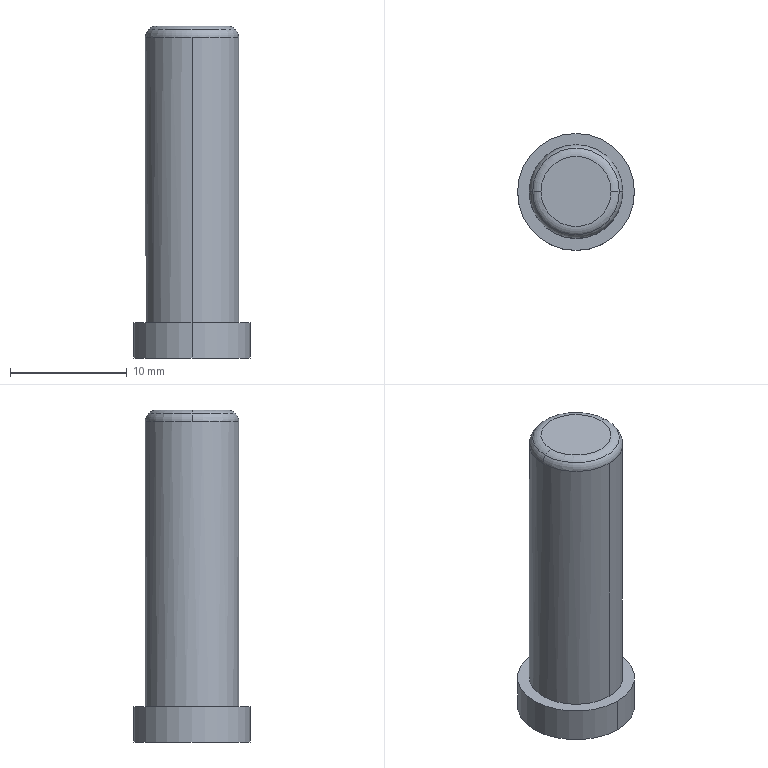Part | STEP file | 1_id1574_x_t | 1 solid | 11 faces | box 10 x 10 x 28.4 mm | volume 1507 mm3 | cylinder 4 | torus 4 | plane 3 | commonest cylinder face diameters 8 x2 10 x2
STEP:
#1=CARTESIAN_POINT('',(0.,0.,0.));
#2=DIRECTION('',(0.,0.,1.));
#3=DIRECTION('',(1.,0.,0.));
#4=AXIS2_PLACEMENT_3D('',#1,#2,#3);
#5=CARTESIAN_POINT('',(335.025,87.797,-28.4));
#6=VERTEX_POINT('',#5);
#7=CARTESIAN_POINT('',(335.025,87.797,-25.4));
#8=VERTEX_POINT('',#7);
#9=CARTESIAN_POINT('',(335.025,87.797,-28.4));
#10=DIRECTION('',(0.,0.,1.));
#11=VECTOR('',#10,1.);
#12=LINE('',#9,#11);
#13=CARTESIAN_POINT('',(335.025,92.797,-46.3));
#14=DIRECTION('',(0.,0.,1.));
#15=DIRECTION('',(0.,-1.,0.));
#16=AXIS2_PLACEMENT_3D('',#13,#14,#15);
#17=CYLINDRICAL_SURFACE('',#16,5.);
#18=CARTESIAN_POINT('',(6.283,17.9));
#19=DIRECTION('',(0.,1.));
#20=VECTOR('',#19,1.);
#21=LINE('',#18,#20);
#22=(GEOMETRIC_REPRESENTATION_CONTEXT(2)PARAMETRIC_REPRESENTATION_CONTEXT()REPRESENTATION_CONTEXT('',''));
#23=DEFINITIONAL_REPRESENTATION('',(#21),#22);
#24=PCURVE('',#17,#23);
#25=CARTESIAN_POINT('',(335.025,92.797,-46.3));
#26=DIRECTION('',(0.,0.,1.));
#27=DIRECTION('',(0.,-1.,0.));
#28=AXIS2_PLACEMENT_3D('',#25,#26,#27);
#29=CYLINDRICAL_SURFACE('',#28,5.);
#30=CARTESIAN_POINT('',(0.,17.9));
#31=DIRECTION('',(0.,1.));
#32=VECTOR('',#31,1.);
#33=LINE('',#30,#32);
#34=(GEOMETRIC_REPRESENTATION_CONTEXT(2)PARAMETRIC_REPRESENTATION_CONTEXT()REPRESENTATION_CONTEXT('',''));
#35=DEFINITIONAL_REPRESENTATION('',(#33),#34);
#36=PCURVE('',#29,#35);
#37=SURFACE_CURVE('',#12,(#24,#36),.PCURVE_S1.);
#38=EDGE_CURVE('',#6,#8,#37,.T.);
#39=ORIENTED_EDGE('',*,*,#38,.T.);
#40=CARTESIAN_POINT('',(335.025,97.797,-25.4));
#41=VERTEX_POINT('',#40);
#42=CARTESIAN_POINT('',(335.025,92.797,-25.4));
#43=DIRECTION('',(0.,0.,1.));
#44=DIRECTION('',(0.,1.,0.));
#45=AXIS2_PLACEMENT_3D('',#42,#43,#44);
#46=CIRCLE('',#45,5.);
#47=CARTESIAN_POINT('',(3.142,20.9));
#48=DIRECTION('',(1.,0.));
#49=VECTOR('',#48,1.);
#50=LINE('',#47,#49);
#51=(GEOMETRIC_REPRESENTATION_CONTEXT(2)PARAMETRIC_REPRESENTATION_CONTEXT()REPRESENTATION_CONTEXT('',''));
#52=DEFINITIONAL_REPRESENTATION('',(#50),#51);
#53=PCURVE('',#17,#52);
#54=CARTESIAN_POINT('',(335.025,92.797,-25.4));
#55=DIRECTION('',(0.,0.,1.));
#56=DIRECTION('',(-1.,0.,0.));
#57=AXIS2_PLACEMENT_3D('',#54,#55,#56);
#58=PLANE('',#57);
#59=CARTESIAN_POINT('',(0.,0.));
#60=DIRECTION('',(0.,-1.));
#61=AXIS2_PLACEMENT_2D('',#59,#60);
#62=CIRCLE('',#61,5.);
#63=(GEOMETRIC_REPRESENTATION_CONTEXT(2)PARAMETRIC_REPRESENTATION_CONTEXT()REPRESENTATION_CONTEXT('',''));
#64=DEFINITIONAL_REPRESENTATION('',(#62),#63);
#65=PCURVE('',#58,#64);
#66=SURFACE_CURVE('',#46,(#53,#65),.PCURVE_S1.);
#67=EDGE_CURVE('',#41,#8,#66,.T.);
#68=ORIENTED_EDGE('',*,*,#67,.F.);
#69=CARTESIAN_POINT('',(335.025,97.797,-28.4));
#70=VERTEX_POINT('',#69);
#71=CARTESIAN_POINT('',(335.025,97.797,-28.4));
#72=DIRECTION('',(0.,0.,-1.));
#73=VECTOR('',#72,1.);
#74=LINE('',#71,#73);
#75=CARTESIAN_POINT('',(3.142,17.9));
#76=DIRECTION('',(0.,-1.));
#77=VECTOR('',#76,1.);
#78=LINE('',#75,#77);
#79=(GEOMETRIC_REPRESENTATION_CONTEXT(2)PARAMETRIC_REPRESENTATION_CONTEXT()REPRESENTATION_CONTEXT('',''));
#80=DEFINITIONAL_REPRESENTATION('',(#78),#79);
#81=PCURVE('',#17,#80);
#82=CARTESIAN_POINT('',(3.142,17.9));
#83=DIRECTION('',(0.,-1.));
#84=VECTOR('',#83,1.);
#85=LINE('',#82,#84);
#86=(GEOMETRIC_REPRESENTATION_CONTEXT(2)PARAMETRIC_REPRESENTATION_CONTEXT()REPRESENTATION_CONTEXT('',''));
#87=DEFINITIONAL_REPRESENTATION('',(#85),#86);
#88=PCURVE('',#29,#87);
#89=SURFACE_CURVE('',#74,(#81,#88),.PCURVE_S1.);
#90=EDGE_CURVE('',#41,#70,#89,.T.);
#91=ORIENTED_EDGE('',*,*,#90,.T.);
#92=CARTESIAN_POINT('',(335.025,92.797,-28.4));
#93=DIRECTION('',(0.,0.,-1.));
#94=DIRECTION('',(0.,-1.,0.));
#95=AXIS2_PLACEMENT_3D('',#92,#93,#94);
#96=CIRCLE('',#95,5.);
#97=CARTESIAN_POINT('',(6.283,17.9));
#98=DIRECTION('',(-1.,0.));
#99=VECTOR('',#98,1.);
#100=LINE('',#97,#99);
#101=(GEOMETRIC_REPRESENTATION_CONTEXT(2)PARAMETRIC_REPRESENTATION_CONTEXT()REPRESENTATION_CONTEXT('',''));
#102=DEFINITIONAL_REPRESENTATION('',(#100),#101);
#103=PCURVE('',#17,#102);
#104=CARTESIAN_POINT('',(335.025,92.797,-28.4));
#105=DIRECTION('',(0.,0.,1.));
#106=DIRECTION('',(-1.,0.,0.));
#107=AXIS2_PLACEMENT_3D('',#104,#105,#106);
#108=PLANE('',#107);
#109=CARTESIAN_POINT('',(0.,5.));
#110=CARTESIAN_POINT('',(8.66,5.));
#111=CARTESIAN_POINT('',(4.33,-2.5));
#112=CARTESIAN_POINT('',(0.,-10.));
#113=CARTESIAN_POINT('',(-4.33,-2.5));
#114=CARTESIAN_POINT('',(-8.66,5.));
#115=CARTESIAN_POINT('',(0.,5.));
#116=(BOUNDED_CURVE()B_SPLINE_CURVE(2,(#109,#110,#111,#112,#113,#114,#115),.UNSPECIFIED.,.T.,.F.)B_SPLINE_CURVE_WITH_KNOTS((1,2,2,2,2,1),(-2.094,0.,2.094,4.189,6.283,8.378),.UNSPECIFIED.)CURVE()GEOMETRIC_REPRESENTATION_ITEM()RATIONAL_B_SPLINE_CURVE((1.,0.5,1.,0.5,1.,0.5,1.))REPRESENTATION_ITEM(''));
#117=(GEOMETRIC_REPRESENTATION_CONTEXT(2)PARAMETRIC_REPRESENTATION_CONTEXT()REPRESENTATION_CONTEXT('',''));
#118=DEFINITIONAL_REPRESENTATION('',(#116),#117);
#119=PCURVE('',#108,#118);
#120=SURFACE_CURVE('',#96,(#103,#119),.PCURVE_S1.);
#121=EDGE_CURVE('',#6,#70,#120,.T.);
#122=ORIENTED_EDGE('',*,*,#121,.F.);
#123=EDGE_LOOP('',(#39,#68,#91,#122));
#124=FACE_BOUND('',#123,.T.);
#125=ADVANCED_FACE('',(#124),#17,.T.);
#126=CARTESIAN_POINT('',(335.025,92.797,-28.4));
#127=DIRECTION('',(0.,0.,-1.));
#128=DIRECTION('',(0.,1.,0.));
#129=AXIS2_PLACEMENT_3D('',#126,#127,#128);
#130=CIRCLE('',#129,5.);
#131=CARTESIAN_POINT('',(0.,-5.));
#132=CARTESIAN_POINT('',(-8.66,-5.));
#133=CARTESIAN_POINT('',(-4.33,2.5));
#134=CARTESIAN_POINT('',(0.,10.));
#135=CARTESIAN_POINT('',(4.33,2.5));
#136=CARTESIAN_POINT('',(8.66,-5.));
#137=CARTESIAN_POINT('',(0.,-5.));
#138=(BOUNDED_CURVE()B_SPLINE_CURVE(2,(#131,#132,#133,#134,#135,#136,#137),.UNSPECIFIED.,.T.,.F.)B_SPLINE_CURVE_WITH_KNOTS((1,2,2,2,2,1),(-2.094,0.,2.094,4.189,6.283,8.378),.UNSPECIFIED.)CURVE()GEOMETRIC_REPRESENTATION_ITEM()RATIONAL_B_SPLINE_CURVE((1.,0.5,1.,0.5,1.,0.5,1.))REPRESENTATION_ITEM(''));
#139=(GEOMETRIC_REPRESENTATION_CONTEXT(2)PARAMETRIC_REPRESENTATION_CONTEXT()REPRESENTATION_CONTEXT('',''));
#140=DEFINITIONAL_REPRESENTATION('',(#138),#139);
#141=PCURVE('',#108,#140);
#142=CARTESIAN_POINT('',(3.142,17.9));
#143=DIRECTION('',(-1.,0.));
#144=VECTOR('',#143,1.);
#145=LINE('',#142,#144);
#146=(GEOMETRIC_REPRESENTATION_CONTEXT(2)PARAMETRIC_REPRESENTATION_CONTEXT()REPRESENTATION_CONTEXT('',''));
#147=DEFINITIONAL_REPRESENTATION('',(#145),#146);
#148=PCURVE('',#29,#147);
#149=SURFACE_CURVE('',#130,(#141,#148),.PCURVE_S1.);
#150=EDGE_CURVE('',#70,#6,#149,.T.);
#151=ORIENTED_EDGE('',*,*,#150,.T.);
#152=ORIENTED_EDGE('',*,*,#121,.T.);
#153=EDGE_LOOP('',(#151,#152));
#154=FACE_BOUND('',#153,.T.);
#155=ADVANCED_FACE('',(#154),#108,.F.);
#156=ORIENTED_EDGE('',*,*,#90,.F.);
#157=CARTESIAN_POINT('',(340.025,92.797,-25.4));
#158=VERTEX_POINT('',#157);
#159=CARTESIAN_POINT('',(335.025,92.797,-25.4));
#160=DIRECTION('',(0.,0.,1.));
#161=DIRECTION('',(1.,0.,0.));
#162=AXIS2_PLACEMENT_3D('',#159,#160,#161);
#163=CIRCLE('',#162,5.);
#164=CARTESIAN_POINT('',(1.571,20.9));
#165=DIRECTION('',(1.,0.));
#166=VECTOR('',#165,1.);
#167=LINE('',#164,#166);
#168=(GEOMETRIC_REPRESENTATION_CONTEXT(2)PARAMETRIC_REPRESENTATION_CONTEXT()REPRESENTATION_CONTEXT('',''));
#169=DEFINITIONAL_REPRESENTATION('',(#167),#168);
#170=PCURVE('',#29,#169);
#171=CARTESIAN_POINT('',(0.,0.));
#172=DIRECTION('',(-1.,0.));
#173=AXIS2_PLACEMENT_2D('',#171,#172);
#174=CIRCLE('',#173,5.);
#175=(GEOMETRIC_REPRESENTATION_CONTEXT(2)PARAMETRIC_REPRESENTATION_CONTEXT()REPRESENTATION_CONTEXT('',''));
#176=DEFINITIONAL_REPRESENTATION('',(#174),#175);
#177=PCURVE('',#58,#176);
#178=SURFACE_CURVE('',#163,(#170,#177),.PCURVE_S1.);
#179=EDGE_CURVE('',#158,#41,#178,.T.);
#180=ORIENTED_EDGE('',*,*,#179,.F.);
#181=CARTESIAN_POINT('',(335.025,92.797,-25.4));
#182=DIRECTION('',(0.,0.,1.));
#183=DIRECTION('',(0.,-1.,0.));
#184=AXIS2_PLACEMENT_3D('',#181,#182,#183);
#185=CIRCLE('',#184,5.);
#186=CARTESIAN_POINT('',(0.,20.9));
#187=DIRECTION('',(1.,0.));
#188=VECTOR('',#187,1.);
#189=LINE('',#186,#188);
#190=(GEOMETRIC_REPRESENTATION_CONTEXT(2)PARAMETRIC_REPRESENTATION_CONTEXT()REPRESENTATION_CONTEXT('',''));
#191=DEFINITIONAL_REPRESENTATION('',(#189),#190);
#192=PCURVE('',#29,#191);
#193=CARTESIAN_POINT('',(0.,0.));
#194=DIRECTION('',(0.,1.));
#195=AXIS2_PLACEMENT_2D('',#193,#194);
#196=CIRCLE('',#195,5.);
#197=(GEOMETRIC_REPRESENTATION_CONTEXT(2)PARAMETRIC_REPRESENTATION_CONTEXT()REPRESENTATION_CONTEXT('',''));
#198=DEFINITIONAL_REPRESENTATION('',(#196),#197);
#199=PCURVE('',#58,#198);
#200=SURFACE_CURVE('',#185,(#192,#199),.PCURVE_S1.);
#201=EDGE_CURVE('',#8,#158,#200,.T.);
#202=ORIENTED_EDGE('',*,*,#201,.F.);
#203=ORIENTED_EDGE('',*,*,#38,.F.);
#204=ORIENTED_EDGE('',*,*,#150,.F.);
#205=EDGE_LOOP('',(#156,#180,#202,#203,#204));
#206=FACE_BOUND('',#205,.T.);
#207=ADVANCED_FACE('',(#206),#29,.T.);
#208=ORIENTED_EDGE('',*,*,#179,.T.);
#209=ORIENTED_EDGE('',*,*,#67,.T.);
#210=ORIENTED_EDGE('',*,*,#201,.T.);
#211=EDGE_LOOP('',(#208,#209,#210));
#212=FACE_BOUND('',#211,.T.);
#213=CARTESIAN_POINT('',(335.025,96.797,-25.4));
#214=VERTEX_POINT('',#213);
#215=CARTESIAN_POINT('',(339.025,92.797,-25.4));
#216=VERTEX_POINT('',#215);
#217=CARTESIAN_POINT('',(335.025,92.797,-25.4));
#218=DIRECTION('',(0.,0.,-1.));
#219=DIRECTION('',(0.,1.,0.));
#220=AXIS2_PLACEMENT_3D('',#217,#218,#219);
#221=CIRCLE('',#220,4.);
#222=CARTESIAN_POINT('',(0.,-4.));
#223=CARTESIAN_POINT('',(-6.928,-4.));
#224=CARTESIAN_POINT('',(-3.464,2.));
#225=CARTESIAN_POINT('',(0.,8.));
#226=CARTESIAN_POINT('',(3.464,2.));
#227=CARTESIAN_POINT('',(6.928,-4.));
#228=CARTESIAN_POINT('',(0.,-4.));
#229=(BOUNDED_CURVE()B_SPLINE_CURVE(2,(#222,#223,#224,#225,#226,#227,#228),.UNSPECIFIED.,.T.,.F.)B_SPLINE_CURVE_WITH_KNOTS((1,2,2,2,2,1),(-2.094,0.,2.094,4.189,6.283,8.378),.UNSPECIFIED.)CURVE()GEOMETRIC_REPRESENTATION_ITEM()RATIONAL_B_SPLINE_CURVE((1.,0.5,1.,0.5,1.,0.5,1.))REPRESENTATION_ITEM(''));
#230=(GEOMETRIC_REPRESENTATION_CONTEXT(2)PARAMETRIC_REPRESENTATION_CONTEXT()REPRESENTATION_CONTEXT('',''));
#231=DEFINITIONAL_REPRESENTATION('',(#229),#230);
#232=PCURVE('',#58,#231);
#233=CARTESIAN_POINT('',(335.025,92.797,-46.3));
#234=DIRECTION('',(0.,0.,-1.));
#235=DIRECTION('',(0.,-1.,0.));
#236=AXIS2_PLACEMENT_3D('',#233,#234,#235);
#237=CYLINDRICAL_SURFACE('',#236,4.);
#238=CARTESIAN_POINT('',(3.142,-20.9));
#239=DIRECTION('',(1.,0.));
#240=VECTOR('',#239,1.);
#241=LINE('',#238,#240);
#242=(GEOMETRIC_REPRESENTATION_CONTEXT(2)PARAMETRIC_REPRESENTATION_CONTEXT()REPRESENTATION_CONTEXT('',''));
#243=DEFINITIONAL_REPRESENTATION('',(#241),#242);
#244=PCURVE('',#237,#243);
#245=SURFACE_CURVE('',#221,(#232,#244),.PCURVE_S1.);
#246=EDGE_CURVE('',#214,#216,#245,.T.);
#247=ORIENTED_EDGE('',*,*,#246,.T.);
#248=CARTESIAN_POINT('',(335.025,88.797,-25.4));
#249=VERTEX_POINT('',#248);
#250=CARTESIAN_POINT('',(335.025,92.797,-25.4));
#251=DIRECTION('',(0.,0.,-1.));
#252=DIRECTION('',(1.,0.,0.));
#253=AXIS2_PLACEMENT_3D('',#250,#251,#252);
#254=CIRCLE('',#253,4.);
#255=CARTESIAN_POINT('',(-4.,0.));
#256=CARTESIAN_POINT('',(-4.,6.928));
#257=CARTESIAN_POINT('',(2.,3.464));
#258=CARTESIAN_POINT('',(8.,0.));
#259=CARTESIAN_POINT('',(2.,-3.464));
#260=CARTESIAN_POINT('',(-4.,-6.928));
#261=CARTESIAN_POINT('',(-4.,0.));
#262=(BOUNDED_CURVE()B_SPLINE_CURVE(2,(#255,#256,#257,#258,#259,#260,#261),.UNSPECIFIED.,.T.,.F.)B_SPLINE_CURVE_WITH_KNOTS((1,2,2,2,2,1),(-2.094,0.,2.094,4.189,6.283,8.378),.UNSPECIFIED.)CURVE()GEOMETRIC_REPRESENTATION_ITEM()RATIONAL_B_SPLINE_CURVE((1.,0.5,1.,0.5,1.,0.5,1.))REPRESENTATION_ITEM(''));
#263=(GEOMETRIC_REPRESENTATION_CONTEXT(2)PARAMETRIC_REPRESENTATION_CONTEXT()REPRESENTATION_CONTEXT('',''));
#264=DEFINITIONAL_REPRESENTATION('',(#262),#263);
#265=PCURVE('',#58,#264);
#266=CARTESIAN_POINT('',(4.712,-20.9));
#267=DIRECTION('',(1.,0.));
#268=VECTOR('',#267,1.);
#269=LINE('',#266,#268);
#270=(GEOMETRIC_REPRESENTATION_CONTEXT(2)PARAMETRIC_REPRESENTATION_CONTEXT()REPRESENTATION_CONTEXT('',''));
#271=DEFINITIONAL_REPRESENTATION('',(#269),#270);
#272=PCURVE('',#237,#271);
#273=SURFACE_CURVE('',#254,(#265,#272),.PCURVE_S1.);
#274=EDGE_CURVE('',#216,#249,#273,.T.);
#275=ORIENTED_EDGE('',*,*,#274,.T.);
#276=CARTESIAN_POINT('',(335.025,92.797,-25.4));
#277=DIRECTION('',(0.,0.,-1.));
#278=DIRECTION('',(0.,-1.,0.));
#279=AXIS2_PLACEMENT_3D('',#276,#277,#278);
#280=CIRCLE('',#279,4.);
#281=CARTESIAN_POINT('',(0.,4.));
#282=CARTESIAN_POINT('',(6.928,4.));
#283=CARTESIAN_POINT('',(3.464,-2.));
#284=CARTESIAN_POINT('',(0.,-8.));
#285=CARTESIAN_POINT('',(-3.464,-2.));
#286=CARTESIAN_POINT('',(-6.928,4.));
#287=CARTESIAN_POINT('',(0.,4.));
#288=(BOUNDED_CURVE()B_SPLINE_CURVE(2,(#281,#282,#283,#284,#285,#286,#287),.UNSPECIFIED.,.T.,.F.)B_SPLINE_CURVE_WITH_KNOTS((1,2,2,2,2,1),(-2.094,0.,2.094,4.189,6.283,8.378),.UNSPECIFIED.)CURVE()GEOMETRIC_REPRESENTATION_ITEM()RATIONAL_B_SPLINE_CURVE((1.,0.5,1.,0.5,1.,0.5,1.))REPRESENTATION_ITEM(''));
#289=(GEOMETRIC_REPRESENTATION_CONTEXT(2)PARAMETRIC_REPRESENTATION_CONTEXT()REPRESENTATION_CONTEXT('',''));
#290=DEFINITIONAL_REPRESENTATION('',(#288),#289);
#291=PCURVE('',#58,#290);
#292=CARTESIAN_POINT('',(335.025,92.797,-46.3));
#293=DIRECTION('',(0.,0.,-1.));
#294=DIRECTION('',(0.,-1.,0.));
#295=AXIS2_PLACEMENT_3D('',#292,#293,#294);
#296=CYLINDRICAL_SURFACE('',#295,4.);
#297=CARTESIAN_POINT('',(0.,-20.9));
#298=DIRECTION('',(1.,0.));
#299=VECTOR('',#298,1.);
#300=LINE('',#297,#299);
#301=(GEOMETRIC_REPRESENTATION_CONTEXT(2)PARAMETRIC_REPRESENTATION_CONTEXT()REPRESENTATION_CONTEXT('',''));
#302=DEFINITIONAL_REPRESENTATION('',(#300),#301);
#303=PCURVE('',#296,#302);
#304=SURFACE_CURVE('',#280,(#291,#303),.PCURVE_S1.);
#305=EDGE_CURVE('',#249,#214,#304,.T.);
#306=ORIENTED_EDGE('',*,*,#305,.T.);
#307=EDGE_LOOP('',(#247,#275,#306));
#308=FACE_BOUND('',#307,.T.);
#309=ADVANCED_FACE('',(#212,#308),#58,.T.);
#310=CARTESIAN_POINT('',(335.025,88.797,-1.));
#311=VERTEX_POINT('',#310);
#312=CARTESIAN_POINT('',(335.025,88.797,-1.));
#313=DIRECTION('',(0.,0.,1.));
#314=VECTOR('',#313,1.);
#315=LINE('',#312,#314);
#316=CARTESIAN_POINT('',(0.,-45.3));
#317=DIRECTION('',(0.,-1.));
#318=VECTOR('',#317,1.);
#319=LINE('',#316,#318);
#320=(GEOMETRIC_REPRESENTATION_CONTEXT(2)PARAMETRIC_REPRESENTATION_CONTEXT()REPRESENTATION_CONTEXT('',''));
#321=DEFINITIONAL_REPRESENTATION('',(#319),#320);
#322=PCURVE('',#296,#321);
#323=CARTESIAN_POINT('',(6.283,-45.3));
#324=DIRECTION('',(0.,-1.));
#325=VECTOR('',#324,1.);
#326=LINE('',#323,#325);
#327=(GEOMETRIC_REPRESENTATION_CONTEXT(2)PARAMETRIC_REPRESENTATION_CONTEXT()REPRESENTATION_CONTEXT('',''));
#328=DEFINITIONAL_REPRESENTATION('',(#326),#327);
#329=PCURVE('',#237,#328);
#330=SURFACE_CURVE('',#315,(#322,#329),.PCURVE_S1.);
#331=EDGE_CURVE('',#249,#311,#330,.T.);
#332=ORIENTED_EDGE('',*,*,#331,.T.);
#333=CARTESIAN_POINT('',(331.025,92.797,-1.));
#334=VERTEX_POINT('',#333);
#335=CARTESIAN_POINT('',(335.025,92.797,-1.));
#336=DIRECTION('',(0.,0.,1.));
#337=DIRECTION('',(-1.,0.,0.));
#338=AXIS2_PLACEMENT_3D('',#335,#336,#337);
#339=CIRCLE('',#338,4.);
#340=CARTESIAN_POINT('',(1.571,-45.3));
#341=DIRECTION('',(-1.,0.));
#342=VECTOR('',#341,1.);
#343=LINE('',#340,#342);
#344=(GEOMETRIC_REPRESENTATION_CONTEXT(2)PARAMETRIC_REPRESENTATION_CONTEXT()REPRESENTATION_CONTEXT('',''));
#345=DEFINITIONAL_REPRESENTATION('',(#343),#344);
#346=PCURVE('',#296,#345);
#347=CARTESIAN_POINT('',(335.025,92.797,-1.));
#348=DIRECTION('',(0.,0.,-1.));
#349=DIRECTION('',(-1.,0.,0.));
#350=AXIS2_PLACEMENT_3D('',#347,#348,#349);
#351=TOROIDAL_SURFACE('',#350,3.,1.);
#352=CARTESIAN_POINT('',(6.283,6.283));
#353=DIRECTION('',(-1.,0.));
#354=VECTOR('',#353,1.);
#355=LINE('',#352,#354);
#356=(GEOMETRIC_REPRESENTATION_CONTEXT(2)PARAMETRIC_REPRESENTATION_CONTEXT()REPRESENTATION_CONTEXT('',''));
#357=DEFINITIONAL_REPRESENTATION('',(#355),#356);
#358=PCURVE('',#351,#357);
#359=SURFACE_CURVE('',#339,(#346,#358),.PCURVE_S1.);
#360=EDGE_CURVE('',#334,#311,#359,.T.);
#361=ORIENTED_EDGE('',*,*,#360,.F.);
#362=CARTESIAN_POINT('',(335.025,96.797,-1.));
#363=VERTEX_POINT('',#362);
#364=CARTESIAN_POINT('',(335.025,92.797,-1.));
#365=DIRECTION('',(0.,0.,1.));
#366=DIRECTION('',(0.,1.,0.));
#367=AXIS2_PLACEMENT_3D('',#364,#365,#366);
#368=CIRCLE('',#367,4.);
#369=CARTESIAN_POINT('',(3.142,-45.3));
#370=DIRECTION('',(-1.,0.));
#371=VECTOR('',#370,1.);
#372=LINE('',#369,#371);
#373=(GEOMETRIC_REPRESENTATION_CONTEXT(2)PARAMETRIC_REPRESENTATION_CONTEXT()REPRESENTATION_CONTEXT('',''));
#374=DEFINITIONAL_REPRESENTATION('',(#372),#373);
#375=PCURVE('',#296,#374);
#376=CARTESIAN_POINT('',(335.025,92.797,-1.));
#377=DIRECTION('',(0.,0.,-1.));
#378=DIRECTION('',(-1.,0.,0.));
#379=AXIS2_PLACEMENT_3D('',#376,#377,#378);
#380=TOROIDAL_SURFACE('',#379,3.,1.);
#381=CARTESIAN_POINT('',(1.571,6.283));
#382=DIRECTION('',(-1.,0.));
#383=VECTOR('',#382,1.);
#384=LINE('',#381,#383);
#385=(GEOMETRIC_REPRESENTATION_CONTEXT(2)PARAMETRIC_REPRESENTATION_CONTEXT()REPRESENTATION_CONTEXT('',''));
#386=DEFINITIONAL_REPRESENTATION('',(#384),#385);
#387=PCURVE('',#380,#386);
#388=SURFACE_CURVE('',#368,(#375,#387),.PCURVE_S1.);
#389=EDGE_CURVE('',#363,#334,#388,.T.);
#390=ORIENTED_EDGE('',*,*,#389,.F.);
#391=CARTESIAN_POINT('',(335.025,96.797,-1.));
#392=DIRECTION('',(0.,0.,-1.));
#393=VECTOR('',#392,1.);
#394=LINE('',#391,#393);
#395=CARTESIAN_POINT('',(3.142,-45.3));
#396=DIRECTION('',(0.,1.));
#397=VECTOR('',#396,1.);
#398=LINE('',#395,#397);
#399=(GEOMETRIC_REPRESENTATION_CONTEXT(2)PARAMETRIC_REPRESENTATION_CONTEXT()REPRESENTATION_CONTEXT('',''));
#400=DEFINITIONAL_REPRESENTATION('',(#398),#399);
#401=PCURVE('',#296,#400);
#402=CARTESIAN_POINT('',(3.142,-45.3));
#403=DIRECTION('',(0.,1.));
#404=VECTOR('',#403,1.);
#405=LINE('',#402,#404);
#406=(GEOMETRIC_REPRESENTATION_CONTEXT(2)PARAMETRIC_REPRESENTATION_CONTEXT()REPRESENTATION_CONTEXT('',''));
#407=DEFINITIONAL_REPRESENTATION('',(#405),#406);
#408=PCURVE('',#237,#407);
#409=SURFACE_CURVE('',#394,(#401,#408),.PCURVE_S1.);
#410=EDGE_CURVE('',#363,#214,#409,.T.);
#411=ORIENTED_EDGE('',*,*,#410,.T.);
#412=ORIENTED_EDGE('',*,*,#305,.F.);
#413=EDGE_LOOP('',(#332,#361,#390,#411,#412));
#414=FACE_BOUND('',#413,.T.);
#415=ADVANCED_FACE('',(#414),#296,.T.);
#416=ORIENTED_EDGE('',*,*,#246,.F.);
#417=ORIENTED_EDGE('',*,*,#410,.F.);
#418=CARTESIAN_POINT('',(339.025,92.797,-1.));
#419=VERTEX_POINT('',#418);
#420=CARTESIAN_POINT('',(335.025,92.797,-1.));
#421=DIRECTION('',(0.,0.,1.));
#422=DIRECTION('',(1.,0.,0.));
#423=AXIS2_PLACEMENT_3D('',#420,#421,#422);
#424=CIRCLE('',#423,4.);
#425=CARTESIAN_POINT('',(4.712,-45.3));
#426=DIRECTION('',(-1.,0.));
#427=VECTOR('',#426,1.);
#428=LINE('',#425,#427);
#429=(GEOMETRIC_REPRESENTATION_CONTEXT(2)PARAMETRIC_REPRESENTATION_CONTEXT()REPRESENTATION_CONTEXT('',''));
#430=DEFINITIONAL_REPRESENTATION('',(#428),#429);
#431=PCURVE('',#237,#430);
#432=CARTESIAN_POINT('',(3.142,6.283));
#433=DIRECTION('',(-1.,0.));
#434=VECTOR('',#433,1.);
#435=LINE('',#432,#434);
#436=(GEOMETRIC_REPRESENTATION_CONTEXT(2)PARAMETRIC_REPRESENTATION_CONTEXT()REPRESENTATION_CONTEXT('',''));
#437=DEFINITIONAL_REPRESENTATION('',(#435),#436);
#438=PCURVE('',#380,#437);
#439=SURFACE_CURVE('',#424,(#431,#438),.PCURVE_S1.);
#440=EDGE_CURVE('',#419,#363,#439,.T.);
#441=ORIENTED_EDGE('',*,*,#440,.F.);
#442=CARTESIAN_POINT('',(335.025,92.797,-1.));
#443=DIRECTION('',(0.,0.,1.));
#444=DIRECTION('',(0.,-1.,0.));
#445=AXIS2_PLACEMENT_3D('',#442,#443,#444);
#446=CIRCLE('',#445,4.);
#447=CARTESIAN_POINT('',(6.283,-45.3));
#448=DIRECTION('',(-1.,0.));
#449=VECTOR('',#448,1.);
#450=LINE('',#447,#449);
#451=(GEOMETRIC_REPRESENTATION_CONTEXT(2)PARAMETRIC_REPRESENTATION_CONTEXT()REPRESENTATION_CONTEXT('',''));
#452=DEFINITIONAL_REPRESENTATION('',(#450),#451);
#453=PCURVE('',#237,#452);
#454=CARTESIAN_POINT('',(4.712,6.283));
#455=DIRECTION('',(-1.,0.));
#456=VECTOR('',#455,1.);
#457=LINE('',#454,#456);
#458=(GEOMETRIC_REPRESENTATION_CONTEXT(2)PARAMETRIC_REPRESENTATION_CONTEXT()REPRESENTATION_CONTEXT('',''));
#459=DEFINITIONAL_REPRESENTATION('',(#457),#458);
#460=PCURVE('',#351,#459);
#461=SURFACE_CURVE('',#446,(#453,#460),.PCURVE_S1.);
#462=EDGE_CURVE('',#311,#419,#461,.T.);
#463=ORIENTED_EDGE('',*,*,#462,.F.);
#464=ORIENTED_EDGE('',*,*,#331,.F.);
#465=ORIENTED_EDGE('',*,*,#274,.F.);
#466=EDGE_LOOP('',(#416,#417,#441,#463,#464,#465));
#467=FACE_BOUND('',#466,.T.);
#468=ADVANCED_FACE('',(#467),#237,.T.);
#469=CARTESIAN_POINT('',(338.732,92.797,-0.2929));
#470=VERTEX_POINT('',#469);
#471=CARTESIAN_POINT('',(338.025,92.797,-1.));
#472=DIRECTION('',(0.,1.,0.));
#473=DIRECTION('',(0.7071,0.,0.7071));
#474=AXIS2_PLACEMENT_3D('',#471,#472,#473);
#475=CIRCLE('',#474,1.);
#476=CARTESIAN_POINT('',(3.142,5.498));
#477=DIRECTION('',(0.,1.));
#478=VECTOR('',#477,1.);
#479=LINE('',#476,#478);
#480=(GEOMETRIC_REPRESENTATION_CONTEXT(2)PARAMETRIC_REPRESENTATION_CONTEXT()REPRESENTATION_CONTEXT('',''));
#481=DEFINITIONAL_REPRESENTATION('',(#479),#480);
#482=PCURVE('',#351,#481);
#483=CARTESIAN_POINT('',(3.142,5.498));
#484=DIRECTION('',(0.,1.));
#485=VECTOR('',#484,1.);
#486=LINE('',#483,#485);
#487=(GEOMETRIC_REPRESENTATION_CONTEXT(2)PARAMETRIC_REPRESENTATION_CONTEXT()REPRESENTATION_CONTEXT('',''));
#488=DEFINITIONAL_REPRESENTATION('',(#486),#487);
#489=PCURVE('',#380,#488);
#490=SURFACE_CURVE('',#475,(#482,#489),.PCURVE_S1.);
#491=EDGE_CURVE('',#470,#419,#490,.T.);
#492=ORIENTED_EDGE('',*,*,#491,.F.);
#493=CARTESIAN_POINT('',(331.318,92.797,-0.2929));
#494=VERTEX_POINT('',#493);
#495=CARTESIAN_POINT('',(335.025,92.797,-0.2929));
#496=DIRECTION('',(0.,0.,-1.));
#497=DIRECTION('',(1.,0.,0.));
#498=AXIS2_PLACEMENT_3D('',#495,#496,#497);
#499=CIRCLE('',#498,3.707);
#500=CARTESIAN_POINT('',(3.142,5.498));
#501=DIRECTION('',(1.,0.));
#502=VECTOR('',#501,1.);
#503=LINE('',#500,#502);
#504=(GEOMETRIC_REPRESENTATION_CONTEXT(2)PARAMETRIC_REPRESENTATION_CONTEXT()REPRESENTATION_CONTEXT('',''));
#505=DEFINITIONAL_REPRESENTATION('',(#503),#504);
#506=PCURVE('',#351,#505);
#507=CARTESIAN_POINT('',(335.025,92.797,-1.));
#508=DIRECTION('',(0.,0.,-1.));
#509=DIRECTION('',(-1.,0.,0.));
#510=AXIS2_PLACEMENT_3D('',#507,#508,#509);
#511=TOROIDAL_SURFACE('',#510,3.,1.);
#512=CARTESIAN_POINT('',(3.142,5.498));
#513=DIRECTION('',(1.,0.));
#514=VECTOR('',#513,1.);
#515=LINE('',#512,#514);
#516=(GEOMETRIC_REPRESENTATION_CONTEXT(2)PARAMETRIC_REPRESENTATION_CONTEXT()REPRESENTATION_CONTEXT('',''));
#517=DEFINITIONAL_REPRESENTATION('',(#515),#516);
#518=PCURVE('',#511,#517);
#519=SURFACE_CURVE('',#499,(#506,#518),.PCURVE_S1.);
#520=EDGE_CURVE('',#470,#494,#519,.T.);
#521=ORIENTED_EDGE('',*,*,#520,.T.);
#522=CARTESIAN_POINT('',(332.025,92.797,-1.));
#523=DIRECTION('',(0.,1.,0.));
#524=DIRECTION('',(-0.7071,0.,0.7071));
#525=AXIS2_PLACEMENT_3D('',#522,#523,#524);
#526=CIRCLE('',#525,1.);
#527=CARTESIAN_POINT('',(6.283,11.781));
#528=DIRECTION('',(0.,-1.));
#529=VECTOR('',#528,1.);
#530=LINE('',#527,#529);
#531=(GEOMETRIC_REPRESENTATION_CONTEXT(2)PARAMETRIC_REPRESENTATION_CONTEXT()REPRESENTATION_CONTEXT('',''));
#532=DEFINITIONAL_REPRESENTATION('',(#530),#531);
#533=PCURVE('',#351,#532);
#534=CARTESIAN_POINT('',(0.,11.781));
#535=DIRECTION('',(0.,-1.));
#536=VECTOR('',#535,1.);
#537=LINE('',#534,#536);
#538=(GEOMETRIC_REPRESENTATION_CONTEXT(2)PARAMETRIC_REPRESENTATION_CONTEXT()REPRESENTATION_CONTEXT('',''));
#539=DEFINITIONAL_REPRESENTATION('',(#537),#538);
#540=PCURVE('',#380,#539);
#541=SURFACE_CURVE('',#526,(#533,#540),.PCURVE_S1.);
#542=EDGE_CURVE('',#334,#494,#541,.T.);
#543=ORIENTED_EDGE('',*,*,#542,.F.);
#544=ORIENTED_EDGE('',*,*,#360,.T.);
#545=ORIENTED_EDGE('',*,*,#462,.T.);
#546=EDGE_LOOP('',(#492,#521,#543,#544,#545));
#547=FACE_BOUND('',#546,.T.);
#548=ADVANCED_FACE('',(#547),#351,.T.);
#549=ORIENTED_EDGE('',*,*,#389,.T.);
#550=ORIENTED_EDGE('',*,*,#542,.T.);
#551=CARTESIAN_POINT('',(335.025,92.797,-0.2929));
#552=DIRECTION('',(0.,0.,-1.));
#553=DIRECTION('',(-1.,0.,0.));
#554=AXIS2_PLACEMENT_3D('',#551,#552,#553);
#555=CIRCLE('',#554,3.707);
#556=CARTESIAN_POINT('',(0.,5.498));
#557=DIRECTION('',(1.,0.));
#558=VECTOR('',#557,1.);
#559=LINE('',#556,#558);
#560=(GEOMETRIC_REPRESENTATION_CONTEXT(2)PARAMETRIC_REPRESENTATION_CONTEXT()REPRESENTATION_CONTEXT('',''));
#561=DEFINITIONAL_REPRESENTATION('',(#559),#560);
#562=PCURVE('',#380,#561);
#563=CARTESIAN_POINT('',(335.025,92.797,-1.));
#564=DIRECTION('',(0.,0.,-1.));
#565=DIRECTION('',(-1.,0.,0.));
#566=AXIS2_PLACEMENT_3D('',#563,#564,#565);
#567=TOROIDAL_SURFACE('',#566,3.,1.);
#568=CARTESIAN_POINT('',(0.,5.498));
#569=DIRECTION('',(1.,0.));
#570=VECTOR('',#569,1.);
#571=LINE('',#568,#570);
#572=(GEOMETRIC_REPRESENTATION_CONTEXT(2)PARAMETRIC_REPRESENTATION_CONTEXT()REPRESENTATION_CONTEXT('',''));
#573=DEFINITIONAL_REPRESENTATION('',(#571),#572);
#574=PCURVE('',#567,#573);
#575=SURFACE_CURVE('',#555,(#562,#574),.PCURVE_S1.);
#576=EDGE_CURVE('',#494,#470,#575,.T.);
#577=ORIENTED_EDGE('',*,*,#576,.T.);
#578=ORIENTED_EDGE('',*,*,#491,.T.);
#579=ORIENTED_EDGE('',*,*,#440,.T.);
#580=EDGE_LOOP('',(#549,#550,#577,#578,#579));
#581=FACE_BOUND('',#580,.T.);
#582=ADVANCED_FACE('',(#581),#380,.T.);
#583=CARTESIAN_POINT('',(338.025,92.797,0.));
#584=VERTEX_POINT('',#583);
#585=CARTESIAN_POINT('',(338.025,92.797,-1.));
#586=DIRECTION('',(0.,1.,0.));
#587=DIRECTION('',(0.,0.,1.));
#588=AXIS2_PLACEMENT_3D('',#585,#586,#587);
#589=CIRCLE('',#588,1.);
#590=CARTESIAN_POINT('',(3.142,4.712));
#591=DIRECTION('',(0.,1.));
#592=VECTOR('',#591,1.);
#593=LINE('',#590,#592);
#594=(GEOMETRIC_REPRESENTATION_CONTEXT(2)PARAMETRIC_REPRESENTATION_CONTEXT()REPRESENTATION_CONTEXT('',''));
#595=DEFINITIONAL_REPRESENTATION('',(#593),#594);
#596=PCURVE('',#567,#595);
#597=CARTESIAN_POINT('',(3.142,4.712));
#598=DIRECTION('',(0.,1.));
#599=VECTOR('',#598,1.);
#600=LINE('',#597,#599);
#601=(GEOMETRIC_REPRESENTATION_CONTEXT(2)PARAMETRIC_REPRESENTATION_CONTEXT()REPRESENTATION_CONTEXT('',''));
#602=DEFINITIONAL_REPRESENTATION('',(#600),#601);
#603=PCURVE('',#511,#602);
#604=SURFACE_CURVE('',#589,(#596,#603),.PCURVE_S1.);
#605=EDGE_CURVE('',#584,#470,#604,.T.);
#606=ORIENTED_EDGE('',*,*,#605,.T.);
#607=ORIENTED_EDGE('',*,*,#576,.F.);
#608=CARTESIAN_POINT('',(332.025,92.797,0.));
#609=VERTEX_POINT('',#608);
#610=CARTESIAN_POINT('',(332.025,92.797,-1.));
#611=DIRECTION('',(0.,1.,0.));
#612=DIRECTION('',(0.,0.,1.));
#613=AXIS2_PLACEMENT_3D('',#610,#611,#612);
#614=CIRCLE('',#613,1.);
#615=CARTESIAN_POINT('',(0.,10.996));
#616=DIRECTION('',(0.,-1.));
#617=VECTOR('',#616,1.);
#618=LINE('',#615,#617);
#619=(GEOMETRIC_REPRESENTATION_CONTEXT(2)PARAMETRIC_REPRESENTATION_CONTEXT()REPRESENTATION_CONTEXT('',''));
#620=DEFINITIONAL_REPRESENTATION('',(#618),#619);
#621=PCURVE('',#567,#620);
#622=CARTESIAN_POINT('',(6.283,10.996));
#623=DIRECTION('',(0.,-1.));
#624=VECTOR('',#623,1.);
#625=LINE('',#622,#624);
#626=(GEOMETRIC_REPRESENTATION_CONTEXT(2)PARAMETRIC_REPRESENTATION_CONTEXT()REPRESENTATION_CONTEXT('',''));
#627=DEFINITIONAL_REPRESENTATION('',(#625),#626);
#628=PCURVE('',#511,#627);
#629=SURFACE_CURVE('',#614,(#621,#628),.PCURVE_S1.);
#630=EDGE_CURVE('',#494,#609,#629,.T.);
#631=ORIENTED_EDGE('',*,*,#630,.T.);
#632=CARTESIAN_POINT('',(335.025,92.797,0.));
#633=DIRECTION('',(0.,0.,1.));
#634=DIRECTION('',(1.,0.,0.));
#635=AXIS2_PLACEMENT_3D('',#632,#633,#634);
#636=CIRCLE('',#635,3.);
#637=CARTESIAN_POINT('',(3.142,4.712));
#638=DIRECTION('',(-1.,0.));
#639=VECTOR('',#638,1.);
#640=LINE('',#637,#639);
#641=(GEOMETRIC_REPRESENTATION_CONTEXT(2)PARAMETRIC_REPRESENTATION_CONTEXT()REPRESENTATION_CONTEXT('',''));
#642=DEFINITIONAL_REPRESENTATION('',(#640),#641);
#643=PCURVE('',#567,#642);
#644=CARTESIAN_POINT('',(335.025,92.797,0.));
#645=DIRECTION('',(0.,0.,-1.));
#646=DIRECTION('',(0.,1.,0.));
#647=AXIS2_PLACEMENT_3D('',#644,#645,#646);
#648=PLANE('',#647);
#649=CARTESIAN_POINT('',(0.,3.));
#650=CARTESIAN_POINT('',(5.196,3.));
#651=CARTESIAN_POINT('',(2.598,-1.5));
#652=CARTESIAN_POINT('',(-0.000000001,-6.));
#653=CARTESIAN_POINT('',(-2.598,-1.5));
#654=CARTESIAN_POINT('',(-5.196,3.));
#655=CARTESIAN_POINT('',(0.,3.));
#656=(BOUNDED_CURVE()B_SPLINE_CURVE(2,(#649,#650,#651,#652,#653,#654,#655),.UNSPECIFIED.,.T.,.F.)B_SPLINE_CURVE_WITH_KNOTS((1,2,2,2,2,1),(-2.094,0.,2.094,4.189,6.283,8.378),.UNSPECIFIED.)CURVE()GEOMETRIC_REPRESENTATION_ITEM()RATIONAL_B_SPLINE_CURVE((1.,0.5,1.,0.5,1.,0.5,1.))REPRESENTATION_ITEM(''));
#657=(GEOMETRIC_REPRESENTATION_CONTEXT(2)PARAMETRIC_REPRESENTATION_CONTEXT()REPRESENTATION_CONTEXT('',''));
#658=DEFINITIONAL_REPRESENTATION('',(#656),#657);
#659=PCURVE('',#648,#658);
#660=SURFACE_CURVE('',#636,(#643,#659),.PCURVE_S1.);
#661=EDGE_CURVE('',#584,#609,#660,.T.);
#662=ORIENTED_EDGE('',*,*,#661,.F.);
#663=EDGE_LOOP('',(#606,#607,#631,#662));
#664=FACE_BOUND('',#663,.T.);
#665=ADVANCED_FACE('',(#664),#567,.T.);
#666=CARTESIAN_POINT('',(335.025,89.797,0.));
#667=VERTEX_POINT('',#666);
#668=CARTESIAN_POINT('',(335.025,92.797,0.));
#669=DIRECTION('',(0.,0.,1.));
#670=DIRECTION('',(-1.,0.,0.));
#671=AXIS2_PLACEMENT_3D('',#668,#669,#670);
#672=CIRCLE('',#671,3.);
#673=CARTESIAN_POINT('',(0.,-3.));
#674=CARTESIAN_POINT('',(-5.196,-3.));
#675=CARTESIAN_POINT('',(-2.598,1.5));
#676=CARTESIAN_POINT('',(0.,6.));
#677=CARTESIAN_POINT('',(2.598,1.5));
#678=CARTESIAN_POINT('',(5.196,-3.));
#679=CARTESIAN_POINT('',(0.,-3.));
#680=(BOUNDED_CURVE()B_SPLINE_CURVE(2,(#673,#674,#675,#676,#677,#678,#679),.UNSPECIFIED.,.T.,.F.)B_SPLINE_CURVE_WITH_KNOTS((1,2,2,2,2,1),(-2.094,0.,2.094,4.189,6.283,8.378),.UNSPECIFIED.)CURVE()GEOMETRIC_REPRESENTATION_ITEM()RATIONAL_B_SPLINE_CURVE((1.,0.5,1.,0.5,1.,0.5,1.))REPRESENTATION_ITEM(''));
#681=(GEOMETRIC_REPRESENTATION_CONTEXT(2)PARAMETRIC_REPRESENTATION_CONTEXT()REPRESENTATION_CONTEXT('',''));
#682=DEFINITIONAL_REPRESENTATION('',(#680),#681);
#683=PCURVE('',#648,#682);
#684=CARTESIAN_POINT('',(6.283,4.712));
#685=DIRECTION('',(-1.,0.));
#686=VECTOR('',#685,1.);
#687=LINE('',#684,#686);
#688=(GEOMETRIC_REPRESENTATION_CONTEXT(2)PARAMETRIC_REPRESENTATION_CONTEXT()REPRESENTATION_CONTEXT('',''));
#689=DEFINITIONAL_REPRESENTATION('',(#687),#688);
#690=PCURVE('',#511,#689);
#691=SURFACE_CURVE('',#672,(#683,#690),.PCURVE_S1.);
#692=EDGE_CURVE('',#609,#667,#691,.T.);
#693=ORIENTED_EDGE('',*,*,#692,.T.);
#694=CARTESIAN_POINT('',(335.025,92.797,0.));
#695=DIRECTION('',(0.,0.,1.));
#696=DIRECTION('',(0.,-1.,0.));
#697=AXIS2_PLACEMENT_3D('',#694,#695,#696);
#698=CIRCLE('',#697,3.);
#699=CARTESIAN_POINT('',(-3.,0.));
#700=CARTESIAN_POINT('',(-3.,5.196));
#701=CARTESIAN_POINT('',(1.5,2.598));
#702=CARTESIAN_POINT('',(6.,0.));
#703=CARTESIAN_POINT('',(1.5,-2.598));
#704=CARTESIAN_POINT('',(-3.,-5.196));
#705=CARTESIAN_POINT('',(-3.,0.));
#706=(BOUNDED_CURVE()B_SPLINE_CURVE(2,(#699,#700,#701,#702,#703,#704,#705),.UNSPECIFIED.,.T.,.F.)B_SPLINE_CURVE_WITH_KNOTS((1,2,2,2,2,1),(-2.094,0.,2.094,4.189,6.283,8.378),.UNSPECIFIED.)CURVE()GEOMETRIC_REPRESENTATION_ITEM()RATIONAL_B_SPLINE_CURVE((1.,0.5,1.,0.5,1.,0.5,1.))REPRESENTATION_ITEM(''));
#707=(GEOMETRIC_REPRESENTATION_CONTEXT(2)PARAMETRIC_REPRESENTATION_CONTEXT()REPRESENTATION_CONTEXT('',''));
#708=DEFINITIONAL_REPRESENTATION('',(#706),#707);
#709=PCURVE('',#648,#708);
#710=CARTESIAN_POINT('',(4.712,4.712));
#711=DIRECTION('',(-1.,0.));
#712=VECTOR('',#711,1.);
#713=LINE('',#710,#712);
#714=(GEOMETRIC_REPRESENTATION_CONTEXT(2)PARAMETRIC_REPRESENTATION_CONTEXT()REPRESENTATION_CONTEXT('',''));
#715=DEFINITIONAL_REPRESENTATION('',(#713),#714);
#716=PCURVE('',#511,#715);
#717=SURFACE_CURVE('',#698,(#709,#716),.PCURVE_S1.);
#718=EDGE_CURVE('',#667,#584,#717,.T.);
#719=ORIENTED_EDGE('',*,*,#718,.T.);
#720=ORIENTED_EDGE('',*,*,#661,.T.);
#721=EDGE_LOOP('',(#693,#719,#720));
#722=FACE_BOUND('',#721,.T.);
#723=ADVANCED_FACE('',(#722),#648,.F.);
#724=ORIENTED_EDGE('',*,*,#630,.F.);
#725=ORIENTED_EDGE('',*,*,#520,.F.);
#726=ORIENTED_EDGE('',*,*,#605,.F.);
#727=ORIENTED_EDGE('',*,*,#718,.F.);
#728=ORIENTED_EDGE('',*,*,#692,.F.);
#729=EDGE_LOOP('',(#724,#725,#726,#727,#728));
#730=FACE_BOUND('',#729,.T.);
#731=ADVANCED_FACE('',(#730),#511,.T.);
#732=CLOSED_SHELL('',(#125,#155,#207,#309,#415,#468,#548,#582,#665,#723,#731));
#733=MANIFOLD_SOLID_BREP('',#732);
#734=(LENGTH_UNIT()NAMED_UNIT(*)SI_UNIT(.MILLI.,.METRE.));
#735=UNCERTAINTY_MEASURE_WITH_UNIT(LENGTH_MEASURE(0.0000001),#734,'','');
#736=(NAMED_UNIT(*)PLANE_ANGLE_UNIT()SI_UNIT($,.RADIAN.));
#737=(NAMED_UNIT(*)SI_UNIT($,.STERADIAN.)SOLID_ANGLE_UNIT());
#738=(GEOMETRIC_REPRESENTATION_CONTEXT(3)GLOBAL_UNCERTAINTY_ASSIGNED_CONTEXT((#735))GLOBAL_UNIT_ASSIGNED_CONTEXT((#734,#736,#737))REPRESENTATION_CONTEXT('',''));
#739=ADVANCED_BREP_SHAPE_REPRESENTATION('',(#4,#733),#738);